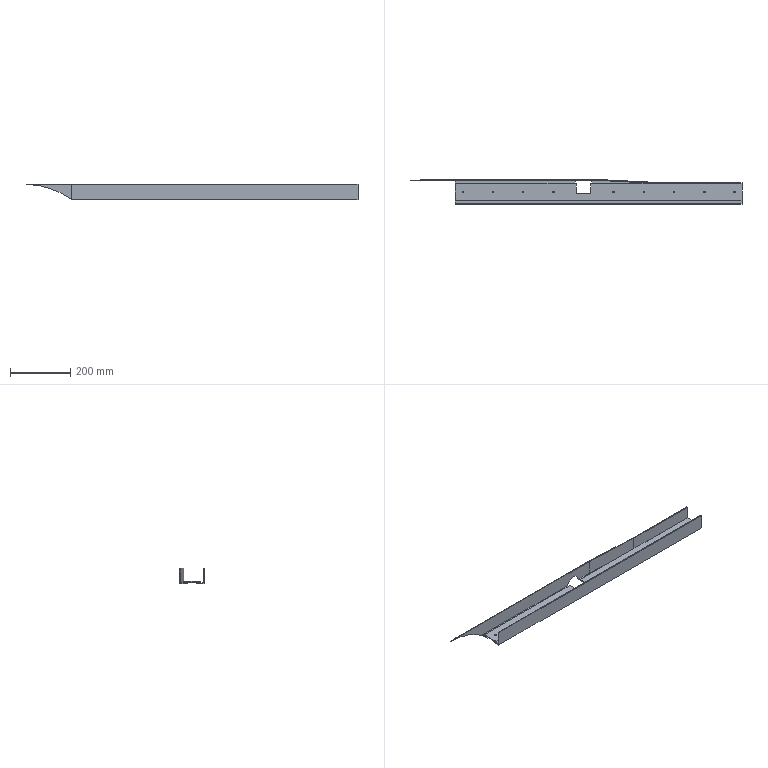Part | SolidWorks | features BaseBody 1 | 1 solid | 50 faces | box 1100 x 80 x 50 mm | volume 549020 mm3 | plane 30 | cylinder 19 | torus 1 | commonest cylinder face diameters 5 x18 50 x1